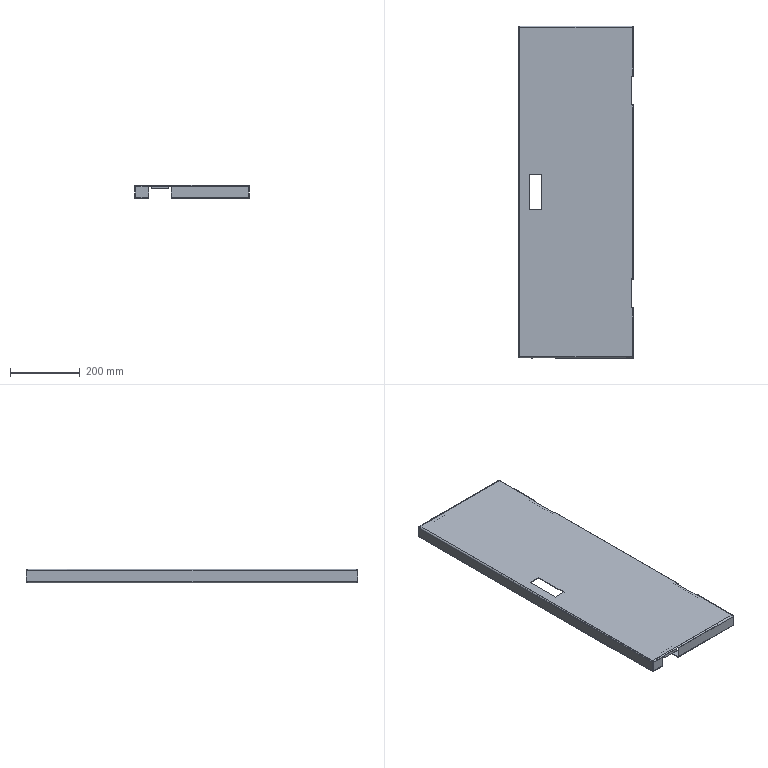Part | SolidWorks | features ICE 5, SMWeldBead 4, Chamfer 2, EdgeFlange 2, HoleWzd 2, FlatPattern 1, SMBaseFlange 1, SheetMetal 1 | 5 solids | 222 faces | box 330 x 954 x 38 mm | volume 933994 mm3 | plane 140 | cylinder 42 | spline 40 | commonest cylinder face diameters 4 x16 8 x14 5 x8 2 x4